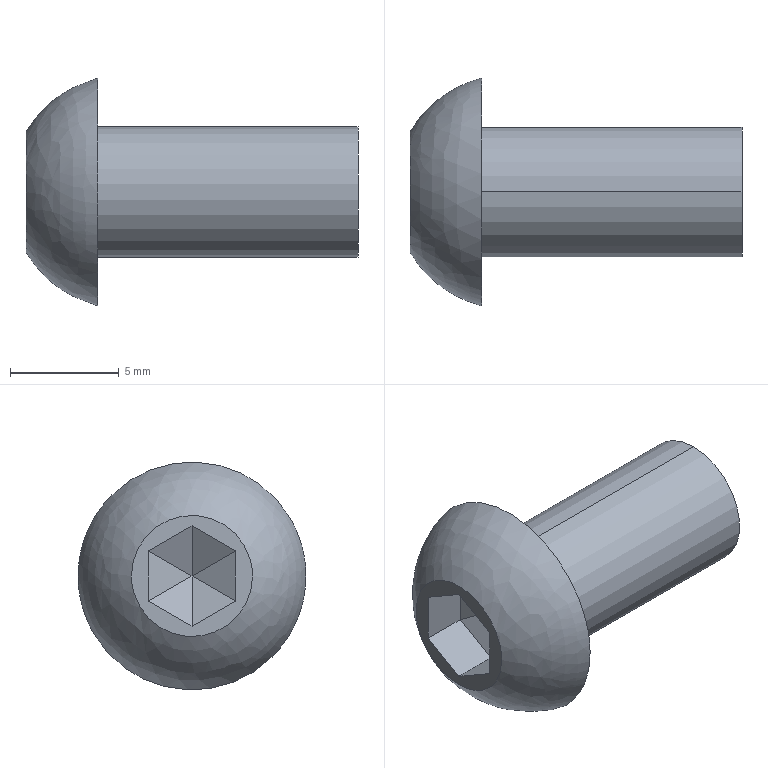Part | STEP file | hexagon socket button head screws_gb_GB_SOCKET_TYPE7 M6X12-N | 1 solid | 18 faces | box 15.3 x 10.5 x 10.5 mm | volume 507.176 mm3 | plane 15 | cylinder 2 | spline 1 | commonest cylinder face diameters 6 x2